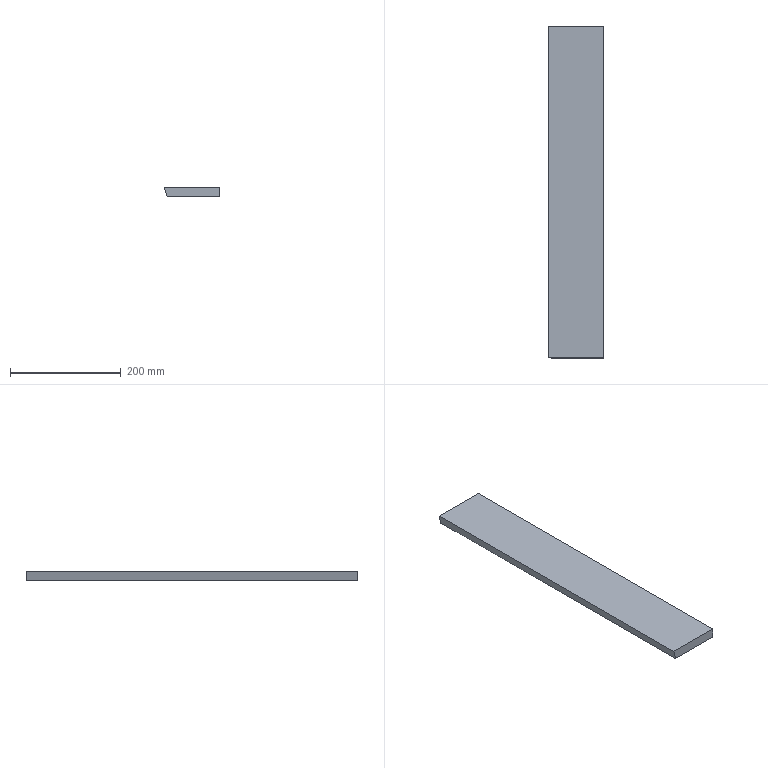Part | STEP file | Leg_left | 1 solid | 6 faces | box 100 x 600 x 18 mm | volume 1053955 mm3 | plane 6
STEP:
#1=CARTESIAN_POINT('',(0.,0.,0.));
#2=DIRECTION('',(0.,0.,1.));
#3=DIRECTION('',(1.,0.,0.));
#4=AXIS2_PLACEMENT_3D('',#1,#2,#3);
#5=CARTESIAN_POINT('',(-45.177,300.,-9.));
#6=VERTEX_POINT('',#5);
#7=CARTESIAN_POINT('',(50.,300.,-9.));
#8=VERTEX_POINT('',#7);
#9=CARTESIAN_POINT('',(-50.,300.,-9.));
#10=DIRECTION('',(1.,0.,0.));
#11=VECTOR('',#10,1.);
#12=LINE('',#9,#11);
#13=CARTESIAN_POINT('',(-50.,300.,-9.));
#14=DIRECTION('',(0.,0.,1.));
#15=DIRECTION('',(1.,0.,0.));
#16=AXIS2_PLACEMENT_3D('',#13,#14,#15);
#17=PLANE('',#16);
#18=CARTESIAN_POINT('',(0.,0.));
#19=DIRECTION('',(1.,0.));
#20=VECTOR('',#19,1.);
#21=LINE('',#18,#20);
#22=(GEOMETRIC_REPRESENTATION_CONTEXT(2)PARAMETRIC_REPRESENTATION_CONTEXT()REPRESENTATION_CONTEXT('',''));
#23=DEFINITIONAL_REPRESENTATION('',(#21),#22);
#24=PCURVE('',#17,#23);
#25=CARTESIAN_POINT('',(0.,300.,0.));
#26=DIRECTION('',(0.,1.,0.));
#27=DIRECTION('',(0.,0.,1.));
#28=AXIS2_PLACEMENT_3D('',#25,#26,#27);
#29=PLANE('',#28);
#30=CARTESIAN_POINT('',(-9.,-50.));
#31=DIRECTION('',(0.,1.));
#32=VECTOR('',#31,1.);
#33=LINE('',#30,#32);
#34=(GEOMETRIC_REPRESENTATION_CONTEXT(2)PARAMETRIC_REPRESENTATION_CONTEXT()REPRESENTATION_CONTEXT('',''));
#35=DEFINITIONAL_REPRESENTATION('',(#33),#34);
#36=PCURVE('',#29,#35);
#37=SURFACE_CURVE('',#12,(#24,#36),.PCURVE_S1.);
#38=EDGE_CURVE('',#6,#8,#37,.T.);
#39=ORIENTED_EDGE('',*,*,#38,.F.);
#40=CARTESIAN_POINT('',(-45.177,-300.,-9.));
#41=VERTEX_POINT('',#40);
#42=CARTESIAN_POINT('',(-45.177,-300.,-9.));
#43=DIRECTION('',(0.,1.,0.));
#44=VECTOR('',#43,1.);
#45=LINE('',#42,#44);
#46=CARTESIAN_POINT('',(4.823,-600.));
#47=DIRECTION('',(0.,1.));
#48=VECTOR('',#47,1.);
#49=LINE('',#46,#48);
#50=(GEOMETRIC_REPRESENTATION_CONTEXT(2)PARAMETRIC_REPRESENTATION_CONTEXT()REPRESENTATION_CONTEXT('',''));
#51=DEFINITIONAL_REPRESENTATION('',(#49),#50);
#52=PCURVE('',#17,#51);
#53=CARTESIAN_POINT('',(-50.,-300.,9.));
#54=DIRECTION('',(-0.9659,0.,-0.2588));
#55=DIRECTION('',(0.2588,0.,-0.9659));
#56=AXIS2_PLACEMENT_3D('',#53,#54,#55);
#57=PLANE('',#56);
#58=CARTESIAN_POINT('',(18.635,0.));
#59=DIRECTION('',(0.,-1.));
#60=VECTOR('',#59,1.);
#61=LINE('',#58,#60);
#62=(GEOMETRIC_REPRESENTATION_CONTEXT(2)PARAMETRIC_REPRESENTATION_CONTEXT()REPRESENTATION_CONTEXT('',''));
#63=DEFINITIONAL_REPRESENTATION('',(#61),#62);
#64=PCURVE('',#57,#63);
#65=SURFACE_CURVE('',#45,(#52,#64),.PCURVE_S1.);
#66=EDGE_CURVE('',#41,#6,#65,.T.);
#67=ORIENTED_EDGE('',*,*,#66,.F.);
#68=CARTESIAN_POINT('',(50.,-300.,-9.));
#69=VERTEX_POINT('',#68);
#70=CARTESIAN_POINT('',(-50.,-300.,-9.));
#71=DIRECTION('',(1.,0.,0.));
#72=VECTOR('',#71,1.);
#73=LINE('',#70,#72);
#74=CARTESIAN_POINT('',(0.,-600.));
#75=DIRECTION('',(1.,0.));
#76=VECTOR('',#75,1.);
#77=LINE('',#74,#76);
#78=(GEOMETRIC_REPRESENTATION_CONTEXT(2)PARAMETRIC_REPRESENTATION_CONTEXT()REPRESENTATION_CONTEXT('',''));
#79=DEFINITIONAL_REPRESENTATION('',(#77),#78);
#80=PCURVE('',#17,#79);
#81=CARTESIAN_POINT('',(0.,-300.,0.));
#82=DIRECTION('',(0.,1.,0.));
#83=DIRECTION('',(0.,0.,1.));
#84=AXIS2_PLACEMENT_3D('',#81,#82,#83);
#85=PLANE('',#84);
#86=CARTESIAN_POINT('',(-9.,-50.));
#87=DIRECTION('',(0.,1.));
#88=VECTOR('',#87,1.);
#89=LINE('',#86,#88);
#90=(GEOMETRIC_REPRESENTATION_CONTEXT(2)PARAMETRIC_REPRESENTATION_CONTEXT()REPRESENTATION_CONTEXT('',''));
#91=DEFINITIONAL_REPRESENTATION('',(#89),#90);
#92=PCURVE('',#85,#91);
#93=SURFACE_CURVE('',#73,(#80,#92),.PCURVE_S1.);
#94=EDGE_CURVE('',#41,#69,#93,.T.);
#95=ORIENTED_EDGE('',*,*,#94,.T.);
#96=CARTESIAN_POINT('',(50.,300.,-9.));
#97=DIRECTION('',(0.,-1.,0.));
#98=VECTOR('',#97,1.);
#99=LINE('',#96,#98);
#100=CARTESIAN_POINT('',(100.,0.));
#101=DIRECTION('',(0.,-1.));
#102=VECTOR('',#101,1.);
#103=LINE('',#100,#102);
#104=(GEOMETRIC_REPRESENTATION_CONTEXT(2)PARAMETRIC_REPRESENTATION_CONTEXT()REPRESENTATION_CONTEXT('',''));
#105=DEFINITIONAL_REPRESENTATION('',(#103),#104);
#106=PCURVE('',#17,#105);
#107=CARTESIAN_POINT('',(50.,300.,-9.));
#108=DIRECTION('',(-1.,0.,0.));
#109=DIRECTION('',(0.,0.,1.));
#110=AXIS2_PLACEMENT_3D('',#107,#108,#109);
#111=PLANE('',#110);
#112=CARTESIAN_POINT('',(0.,0.));
#113=DIRECTION('',(0.,-1.));
#114=VECTOR('',#113,1.);
#115=LINE('',#112,#114);
#116=(GEOMETRIC_REPRESENTATION_CONTEXT(2)PARAMETRIC_REPRESENTATION_CONTEXT()REPRESENTATION_CONTEXT('',''));
#117=DEFINITIONAL_REPRESENTATION('',(#115),#116);
#118=PCURVE('',#111,#117);
#119=SURFACE_CURVE('',#99,(#106,#118),.PCURVE_S1.);
#120=EDGE_CURVE('',#8,#69,#119,.T.);
#121=ORIENTED_EDGE('',*,*,#120,.F.);
#122=EDGE_LOOP('',(#39,#67,#95,#121));
#123=FACE_BOUND('',#122,.F.);
#124=ADVANCED_FACE('',(#123),#17,.F.);
#125=ORIENTED_EDGE('',*,*,#38,.F.);
#126=CARTESIAN_POINT('',(-50.,300.,9.));
#127=VERTEX_POINT('',#126);
#128=CARTESIAN_POINT('',(-47.2,300.,-1.449));
#129=DIRECTION('',(0.2588,0.,-0.9659));
#130=VECTOR('',#129,1.);
#131=LINE('',#128,#130);
#132=CARTESIAN_POINT('',(-1.449,-47.2));
#133=DIRECTION('',(-0.9659,0.2588));
#134=VECTOR('',#133,1.);
#135=LINE('',#132,#134);
#136=(GEOMETRIC_REPRESENTATION_CONTEXT(2)PARAMETRIC_REPRESENTATION_CONTEXT()REPRESENTATION_CONTEXT('',''));
#137=DEFINITIONAL_REPRESENTATION('',(#135),#136);
#138=PCURVE('',#29,#137);
#139=CARTESIAN_POINT('',(10.817,-600.));
#140=DIRECTION('',(1.,0.));
#141=VECTOR('',#140,1.);
#142=LINE('',#139,#141);
#143=(GEOMETRIC_REPRESENTATION_CONTEXT(2)PARAMETRIC_REPRESENTATION_CONTEXT()REPRESENTATION_CONTEXT('',''));
#144=DEFINITIONAL_REPRESENTATION('',(#142),#143);
#145=PCURVE('',#57,#144);
#146=SURFACE_CURVE('',#131,(#138,#145),.PCURVE_S1.);
#147=EDGE_CURVE('',#127,#6,#146,.T.);
#148=ORIENTED_EDGE('',*,*,#147,.F.);
#149=CARTESIAN_POINT('',(50.,300.,9.));
#150=VERTEX_POINT('',#149);
#151=CARTESIAN_POINT('',(50.,300.,9.));
#152=DIRECTION('',(-1.,0.,0.));
#153=VECTOR('',#152,1.);
#154=LINE('',#151,#153);
#155=CARTESIAN_POINT('',(9.,50.));
#156=DIRECTION('',(0.,-1.));
#157=VECTOR('',#156,1.);
#158=LINE('',#155,#157);
#159=(GEOMETRIC_REPRESENTATION_CONTEXT(2)PARAMETRIC_REPRESENTATION_CONTEXT()REPRESENTATION_CONTEXT('',''));
#160=DEFINITIONAL_REPRESENTATION('',(#158),#159);
#161=PCURVE('',#29,#160);
#162=CARTESIAN_POINT('',(50.,300.,9.));
#163=DIRECTION('',(0.,0.,-1.));
#164=DIRECTION('',(-1.,0.,0.));
#165=AXIS2_PLACEMENT_3D('',#162,#163,#164);
#166=PLANE('',#165);
#167=CARTESIAN_POINT('',(0.,0.));
#168=DIRECTION('',(1.,0.));
#169=VECTOR('',#168,1.);
#170=LINE('',#167,#169);
#171=(GEOMETRIC_REPRESENTATION_CONTEXT(2)PARAMETRIC_REPRESENTATION_CONTEXT()REPRESENTATION_CONTEXT('',''));
#172=DEFINITIONAL_REPRESENTATION('',(#170),#171);
#173=PCURVE('',#166,#172);
#174=SURFACE_CURVE('',#154,(#161,#173),.PCURVE_S1.);
#175=EDGE_CURVE('',#150,#127,#174,.T.);
#176=ORIENTED_EDGE('',*,*,#175,.F.);
#177=CARTESIAN_POINT('',(50.,300.,-9.));
#178=DIRECTION('',(0.,0.,1.));
#179=VECTOR('',#178,1.);
#180=LINE('',#177,#179);
#181=CARTESIAN_POINT('',(-9.,50.));
#182=DIRECTION('',(1.,0.));
#183=VECTOR('',#182,1.);
#184=LINE('',#181,#183);
#185=(GEOMETRIC_REPRESENTATION_CONTEXT(2)PARAMETRIC_REPRESENTATION_CONTEXT()REPRESENTATION_CONTEXT('',''));
#186=DEFINITIONAL_REPRESENTATION('',(#184),#185);
#187=PCURVE('',#29,#186);
#188=CARTESIAN_POINT('',(0.,0.));
#189=DIRECTION('',(1.,0.));
#190=VECTOR('',#189,1.);
#191=LINE('',#188,#190);
#192=(GEOMETRIC_REPRESENTATION_CONTEXT(2)PARAMETRIC_REPRESENTATION_CONTEXT()REPRESENTATION_CONTEXT('',''));
#193=DEFINITIONAL_REPRESENTATION('',(#191),#192);
#194=PCURVE('',#111,#193);
#195=SURFACE_CURVE('',#180,(#187,#194),.PCURVE_S1.);
#196=EDGE_CURVE('',#8,#150,#195,.T.);
#197=ORIENTED_EDGE('',*,*,#196,.F.);
#198=EDGE_LOOP('',(#125,#148,#176,#197));
#199=FACE_BOUND('',#198,.T.);
#200=ADVANCED_FACE('',(#199),#29,.T.);
#201=ORIENTED_EDGE('',*,*,#120,.T.);
#202=CARTESIAN_POINT('',(50.,-300.,9.));
#203=VERTEX_POINT('',#202);
#204=CARTESIAN_POINT('',(50.,-300.,-9.));
#205=DIRECTION('',(0.,0.,1.));
#206=VECTOR('',#205,1.);
#207=LINE('',#204,#206);
#208=CARTESIAN_POINT('',(0.,-600.));
#209=DIRECTION('',(1.,0.));
#210=VECTOR('',#209,1.);
#211=LINE('',#208,#210);
#212=(GEOMETRIC_REPRESENTATION_CONTEXT(2)PARAMETRIC_REPRESENTATION_CONTEXT()REPRESENTATION_CONTEXT('',''));
#213=DEFINITIONAL_REPRESENTATION('',(#211),#212);
#214=PCURVE('',#111,#213);
#215=CARTESIAN_POINT('',(-9.,50.));
#216=DIRECTION('',(1.,0.));
#217=VECTOR('',#216,1.);
#218=LINE('',#215,#217);
#219=(GEOMETRIC_REPRESENTATION_CONTEXT(2)PARAMETRIC_REPRESENTATION_CONTEXT()REPRESENTATION_CONTEXT('',''));
#220=DEFINITIONAL_REPRESENTATION('',(#218),#219);
#221=PCURVE('',#85,#220);
#222=SURFACE_CURVE('',#207,(#214,#221),.PCURVE_S1.);
#223=EDGE_CURVE('',#69,#203,#222,.T.);
#224=ORIENTED_EDGE('',*,*,#223,.T.);
#225=CARTESIAN_POINT('',(50.,300.,9.));
#226=DIRECTION('',(0.,-1.,0.));
#227=VECTOR('',#226,1.);
#228=LINE('',#225,#227);
#229=CARTESIAN_POINT('',(18.,0.));
#230=DIRECTION('',(0.,-1.));
#231=VECTOR('',#230,1.);
#232=LINE('',#229,#231);
#233=(GEOMETRIC_REPRESENTATION_CONTEXT(2)PARAMETRIC_REPRESENTATION_CONTEXT()REPRESENTATION_CONTEXT('',''));
#234=DEFINITIONAL_REPRESENTATION('',(#232),#233);
#235=PCURVE('',#111,#234);
#236=CARTESIAN_POINT('',(0.,0.));
#237=DIRECTION('',(0.,-1.));
#238=VECTOR('',#237,1.);
#239=LINE('',#236,#238);
#240=(GEOMETRIC_REPRESENTATION_CONTEXT(2)PARAMETRIC_REPRESENTATION_CONTEXT()REPRESENTATION_CONTEXT('',''));
#241=DEFINITIONAL_REPRESENTATION('',(#239),#240);
#242=PCURVE('',#166,#241);
#243=SURFACE_CURVE('',#228,(#235,#242),.PCURVE_S1.);
#244=EDGE_CURVE('',#150,#203,#243,.T.);
#245=ORIENTED_EDGE('',*,*,#244,.F.);
#246=ORIENTED_EDGE('',*,*,#196,.F.);
#247=EDGE_LOOP('',(#201,#224,#245,#246));
#248=FACE_BOUND('',#247,.F.);
#249=ADVANCED_FACE('',(#248),#111,.F.);
#250=ORIENTED_EDGE('',*,*,#94,.F.);
#251=CARTESIAN_POINT('',(-50.,-300.,9.));
#252=VERTEX_POINT('',#251);
#253=CARTESIAN_POINT('',(-50.,-300.,9.));
#254=DIRECTION('',(0.2588,0.,-0.9659));
#255=VECTOR('',#254,1.);
#256=LINE('',#253,#255);
#257=CARTESIAN_POINT('',(9.,-50.));
#258=DIRECTION('',(-0.9659,0.2588));
#259=VECTOR('',#258,1.);
#260=LINE('',#257,#259);
#261=(GEOMETRIC_REPRESENTATION_CONTEXT(2)PARAMETRIC_REPRESENTATION_CONTEXT()REPRESENTATION_CONTEXT('',''));
#262=DEFINITIONAL_REPRESENTATION('',(#260),#261);
#263=PCURVE('',#85,#262);
#264=CARTESIAN_POINT('',(0.,0.));
#265=DIRECTION('',(1.,0.));
#266=VECTOR('',#265,1.);
#267=LINE('',#264,#266);
#268=(GEOMETRIC_REPRESENTATION_CONTEXT(2)PARAMETRIC_REPRESENTATION_CONTEXT()REPRESENTATION_CONTEXT('',''));
#269=DEFINITIONAL_REPRESENTATION('',(#267),#268);
#270=PCURVE('',#57,#269);
#271=SURFACE_CURVE('',#256,(#263,#270),.PCURVE_S1.);
#272=EDGE_CURVE('',#252,#41,#271,.T.);
#273=ORIENTED_EDGE('',*,*,#272,.F.);
#274=CARTESIAN_POINT('',(50.,-300.,9.));
#275=DIRECTION('',(-1.,0.,0.));
#276=VECTOR('',#275,1.);
#277=LINE('',#274,#276);
#278=CARTESIAN_POINT('',(9.,50.));
#279=DIRECTION('',(0.,-1.));
#280=VECTOR('',#279,1.);
#281=LINE('',#278,#280);
#282=(GEOMETRIC_REPRESENTATION_CONTEXT(2)PARAMETRIC_REPRESENTATION_CONTEXT()REPRESENTATION_CONTEXT('',''));
#283=DEFINITIONAL_REPRESENTATION('',(#281),#282);
#284=PCURVE('',#85,#283);
#285=CARTESIAN_POINT('',(0.,-600.));
#286=DIRECTION('',(1.,0.));
#287=VECTOR('',#286,1.);
#288=LINE('',#285,#287);
#289=(GEOMETRIC_REPRESENTATION_CONTEXT(2)PARAMETRIC_REPRESENTATION_CONTEXT()REPRESENTATION_CONTEXT('',''));
#290=DEFINITIONAL_REPRESENTATION('',(#288),#289);
#291=PCURVE('',#166,#290);
#292=SURFACE_CURVE('',#277,(#284,#291),.PCURVE_S1.);
#293=EDGE_CURVE('',#203,#252,#292,.T.);
#294=ORIENTED_EDGE('',*,*,#293,.F.);
#295=ORIENTED_EDGE('',*,*,#223,.F.);
#296=EDGE_LOOP('',(#250,#273,#294,#295));
#297=FACE_BOUND('',#296,.F.);
#298=ADVANCED_FACE('',(#297),#85,.F.);
#299=ORIENTED_EDGE('',*,*,#272,.F.);
#300=CARTESIAN_POINT('',(-50.,300.,9.));
#301=DIRECTION('',(0.,-1.,0.));
#302=VECTOR('',#301,1.);
#303=LINE('',#300,#302);
#304=CARTESIAN_POINT('',(0.,-600.));
#305=DIRECTION('',(0.,1.));
#306=VECTOR('',#305,1.);
#307=LINE('',#304,#306);
#308=(GEOMETRIC_REPRESENTATION_CONTEXT(2)PARAMETRIC_REPRESENTATION_CONTEXT()REPRESENTATION_CONTEXT('',''));
#309=DEFINITIONAL_REPRESENTATION('',(#307),#308);
#310=PCURVE('',#57,#309);
#311=CARTESIAN_POINT('',(100.,0.));
#312=DIRECTION('',(0.,-1.));
#313=VECTOR('',#312,1.);
#314=LINE('',#311,#313);
#315=(GEOMETRIC_REPRESENTATION_CONTEXT(2)PARAMETRIC_REPRESENTATION_CONTEXT()REPRESENTATION_CONTEXT('',''));
#316=DEFINITIONAL_REPRESENTATION('',(#314),#315);
#317=PCURVE('',#166,#316);
#318=SURFACE_CURVE('',#303,(#310,#317),.PCURVE_S1.);
#319=EDGE_CURVE('',#127,#252,#318,.T.);
#320=ORIENTED_EDGE('',*,*,#319,.F.);
#321=ORIENTED_EDGE('',*,*,#147,.T.);
#322=ORIENTED_EDGE('',*,*,#66,.F.);
#323=EDGE_LOOP('',(#299,#320,#321,#322));
#324=FACE_BOUND('',#323,.T.);
#325=ADVANCED_FACE('',(#324),#57,.T.);
#326=ORIENTED_EDGE('',*,*,#244,.T.);
#327=ORIENTED_EDGE('',*,*,#293,.T.);
#328=ORIENTED_EDGE('',*,*,#319,.F.);
#329=ORIENTED_EDGE('',*,*,#175,.F.);
#330=EDGE_LOOP('',(#326,#327,#328,#329));
#331=FACE_BOUND('',#330,.F.);
#332=ADVANCED_FACE('',(#331),#166,.F.);
#333=CLOSED_SHELL('',(#124,#200,#249,#298,#325,#332));
#334=MANIFOLD_SOLID_BREP('',#333);
#335=(LENGTH_UNIT()NAMED_UNIT(*)SI_UNIT(.MILLI.,.METRE.));
#336=UNCERTAINTY_MEASURE_WITH_UNIT(LENGTH_MEASURE(0.0000001),#335,'','');
#337=(NAMED_UNIT(*)PLANE_ANGLE_UNIT()SI_UNIT($,.RADIAN.));
#338=(NAMED_UNIT(*)SI_UNIT($,.STERADIAN.)SOLID_ANGLE_UNIT());
#339=(GEOMETRIC_REPRESENTATION_CONTEXT(3)GLOBAL_UNCERTAINTY_ASSIGNED_CONTEXT((#336))GLOBAL_UNIT_ASSIGNED_CONTEXT((#335,#337,#338))REPRESENTATION_CONTEXT('',''));
#340=ADVANCED_BREP_SHAPE_REPRESENTATION('',(#4,#334),#339);